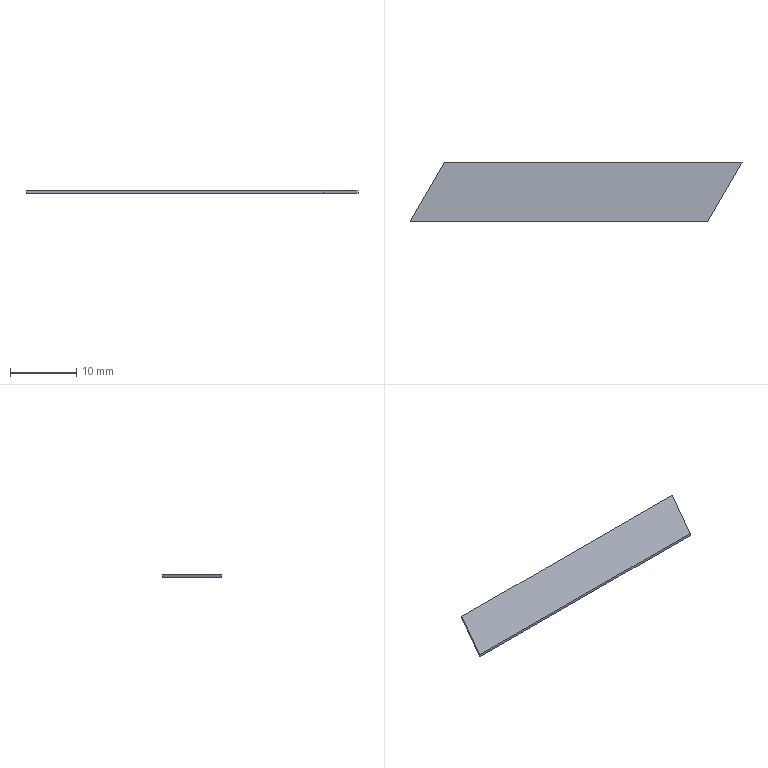Part | SolidWorks | features Extrusion 1 | 1 solid | 6 faces | box 50.196 x 9 x 0.4 mm | volume 162 mm3 | plane 6
STEP:
#1=CARTESIAN_POINT('',(5.196,9.,0.));
#2=VERTEX_POINT('',#1);
#3=CARTESIAN_POINT('',(0.,0.,0.));
#4=VERTEX_POINT('',#3);
#5=CARTESIAN_POINT('',(0.,0.,0.));
#6=DIRECTION('',(-0.5,-0.866,0.));
#7=VECTOR('',#6,1000.);
#8=LINE('',#5,#7);
#9=EDGE_CURVE('',#2,#4,#8,.T.);
#10=ORIENTED_EDGE('',*,*,#9,.T.);
#11=CARTESIAN_POINT('',(0.,0.,0.4));
#12=VERTEX_POINT('',#11);
#13=CARTESIAN_POINT('',(0.,0.,0.4));
#14=DIRECTION('',(0.,0.,-1.));
#15=VECTOR('',#14,1000.);
#16=LINE('',#13,#15);
#17=EDGE_CURVE('',#12,#4,#16,.T.);
#18=ORIENTED_EDGE('',*,*,#17,.F.);
#19=CARTESIAN_POINT('',(5.196,9.,0.4));
#20=VERTEX_POINT('',#19);
#21=CARTESIAN_POINT('',(0.,0.,0.4));
#22=DIRECTION('',(-0.5,-0.866,0.));
#23=VECTOR('',#22,1000.);
#24=LINE('',#21,#23);
#25=EDGE_CURVE('',#20,#12,#24,.T.);
#26=ORIENTED_EDGE('',*,*,#25,.F.);
#27=CARTESIAN_POINT('',(5.196,9.,0.4));
#28=DIRECTION('',(0.,0.,-1.));
#29=VECTOR('',#28,1000.);
#30=LINE('',#27,#29);
#31=EDGE_CURVE('',#20,#2,#30,.T.);
#32=ORIENTED_EDGE('',*,*,#31,.T.);
#33=EDGE_LOOP('',(#10,#18,#26,#32));
#34=FACE_OUTER_BOUND('',#33,.T.);
#35=CARTESIAN_POINT('',(0.,0.,0.4));
#36=DIRECTION('',(0.866,-0.5,0.));
#37=DIRECTION('',(0.5,0.866,0.));
#38=AXIS2_PLACEMENT_3D('',#35,#36,#37);
#39=PLANE('',#38);
#40=ADVANCED_FACE('',(#34),#39,.F.);
#41=CARTESIAN_POINT('',(45.,0.,0.));
#42=VERTEX_POINT('',#41);
#43=CARTESIAN_POINT('',(0.,0.,0.));
#44=DIRECTION('',(1.,0.,0.));
#45=VECTOR('',#44,1000.);
#46=LINE('',#43,#45);
#47=EDGE_CURVE('',#4,#42,#46,.T.);
#48=ORIENTED_EDGE('',*,*,#47,.T.);
#49=CARTESIAN_POINT('',(45.,0.,0.4));
#50=VERTEX_POINT('',#49);
#51=CARTESIAN_POINT('',(45.,0.,0.4));
#52=DIRECTION('',(0.,0.,-1.));
#53=VECTOR('',#52,1000.);
#54=LINE('',#51,#53);
#55=EDGE_CURVE('',#50,#42,#54,.T.);
#56=ORIENTED_EDGE('',*,*,#55,.F.);
#57=CARTESIAN_POINT('',(0.,0.,0.4));
#58=DIRECTION('',(1.,0.,0.));
#59=VECTOR('',#58,1000.);
#60=LINE('',#57,#59);
#61=EDGE_CURVE('',#12,#50,#60,.T.);
#62=ORIENTED_EDGE('',*,*,#61,.F.);
#63=ORIENTED_EDGE('',*,*,#17,.T.);
#64=EDGE_LOOP('',(#48,#56,#62,#63));
#65=FACE_OUTER_BOUND('',#64,.T.);
#66=CARTESIAN_POINT('',(0.,0.,0.4));
#67=DIRECTION('',(0.,1.,0.));
#68=DIRECTION('',(0.,0.,1.));
#69=AXIS2_PLACEMENT_3D('',#66,#67,#68);
#70=PLANE('',#69);
#71=ADVANCED_FACE('',(#65),#70,.F.);
#72=CARTESIAN_POINT('',(50.196,9.,0.));
#73=VERTEX_POINT('',#72);
#74=CARTESIAN_POINT('',(45.,0.,0.));
#75=DIRECTION('',(0.5,0.866,0.));
#76=VECTOR('',#75,1000.);
#77=LINE('',#74,#76);
#78=EDGE_CURVE('',#42,#73,#77,.T.);
#79=ORIENTED_EDGE('',*,*,#78,.T.);
#80=CARTESIAN_POINT('',(50.196,9.,0.4));
#81=VERTEX_POINT('',#80);
#82=CARTESIAN_POINT('',(50.196,9.,0.4));
#83=DIRECTION('',(0.,0.,-1.));
#84=VECTOR('',#83,1000.);
#85=LINE('',#82,#84);
#86=EDGE_CURVE('',#81,#73,#85,.T.);
#87=ORIENTED_EDGE('',*,*,#86,.F.);
#88=CARTESIAN_POINT('',(45.,0.,0.4));
#89=DIRECTION('',(0.5,0.866,0.));
#90=VECTOR('',#89,1000.);
#91=LINE('',#88,#90);
#92=EDGE_CURVE('',#50,#81,#91,.T.);
#93=ORIENTED_EDGE('',*,*,#92,.F.);
#94=ORIENTED_EDGE('',*,*,#55,.T.);
#95=EDGE_LOOP('',(#79,#87,#93,#94));
#96=FACE_OUTER_BOUND('',#95,.T.);
#97=CARTESIAN_POINT('',(45.,0.,0.4));
#98=DIRECTION('',(-0.866,0.5,0.));
#99=DIRECTION('',(-0.5,-0.866,0.));
#100=AXIS2_PLACEMENT_3D('',#97,#98,#99);
#101=PLANE('',#100);
#102=ADVANCED_FACE('',(#96),#101,.F.);
#103=CARTESIAN_POINT('',(5.196,9.,0.));
#104=DIRECTION('',(-1.,0.,0.));
#105=VECTOR('',#104,1000.);
#106=LINE('',#103,#105);
#107=EDGE_CURVE('',#73,#2,#106,.T.);
#108=ORIENTED_EDGE('',*,*,#107,.T.);
#109=ORIENTED_EDGE('',*,*,#31,.F.);
#110=CARTESIAN_POINT('',(5.196,9.,0.4));
#111=DIRECTION('',(-1.,0.,0.));
#112=VECTOR('',#111,1000.);
#113=LINE('',#110,#112);
#114=EDGE_CURVE('',#81,#20,#113,.T.);
#115=ORIENTED_EDGE('',*,*,#114,.F.);
#116=ORIENTED_EDGE('',*,*,#86,.T.);
#117=EDGE_LOOP('',(#108,#109,#115,#116));
#118=FACE_OUTER_BOUND('',#117,.T.);
#119=CARTESIAN_POINT('',(5.196,9.,0.4));
#120=DIRECTION('',(0.,-1.,0.));
#121=DIRECTION('',(0.,0.,-1.));
#122=AXIS2_PLACEMENT_3D('',#119,#120,#121);
#123=PLANE('',#122);
#124=ADVANCED_FACE('',(#118),#123,.F.);
#125=ORIENTED_EDGE('',*,*,#25,.T.);
#126=ORIENTED_EDGE('',*,*,#61,.T.);
#127=ORIENTED_EDGE('',*,*,#92,.T.);
#128=ORIENTED_EDGE('',*,*,#114,.T.);
#129=EDGE_LOOP('',(#125,#126,#127,#128));
#130=FACE_OUTER_BOUND('',#129,.T.);
#131=CARTESIAN_POINT('',(0.,0.,0.4));
#132=DIRECTION('',(0.,0.,-1.));
#133=DIRECTION('',(-1.,0.,0.));
#134=AXIS2_PLACEMENT_3D('',#131,#132,#133);
#135=PLANE('',#134);
#136=ADVANCED_FACE('',(#130),#135,.F.);
#137=ORIENTED_EDGE('',*,*,#9,.F.);
#138=ORIENTED_EDGE('',*,*,#107,.F.);
#139=ORIENTED_EDGE('',*,*,#78,.F.);
#140=ORIENTED_EDGE('',*,*,#47,.F.);
#141=EDGE_LOOP('',(#137,#138,#139,#140));
#142=FACE_OUTER_BOUND('',#141,.T.);
#143=CARTESIAN_POINT('',(0.,0.,0.));
#144=DIRECTION('',(0.,0.,-1.));
#145=DIRECTION('',(-1.,0.,0.));
#146=AXIS2_PLACEMENT_3D('',#143,#144,#145);
#147=PLANE('',#146);
#148=ADVANCED_FACE('',(#142),#147,.T.);
#149=CLOSED_SHELL('',(#40,#71,#102,#124,#136,#148));
#150=MANIFOLD_SOLID_BREP('',#149);
#151=CARTESIAN_POINT('',(0.,0.,0.));
#152=DIRECTION('',(0.,0.,1.));
#153=DIRECTION('',(1.,0.,0.));
#154=AXIS2_PLACEMENT_3D('',#151,#152,#153);
#155=(LENGTH_UNIT()NAMED_UNIT(*)SI_UNIT(.MILLI.,.METRE.));
#156=UNCERTAINTY_MEASURE_WITH_UNIT(LENGTH_MEASURE(0.00001),#155,'','');
#157=(NAMED_UNIT(*)PLANE_ANGLE_UNIT()SI_UNIT($,.RADIAN.));
#158=(NAMED_UNIT(*)SI_UNIT($,.STERADIAN.)SOLID_ANGLE_UNIT());
#159=(GEOMETRIC_REPRESENTATION_CONTEXT(3)GLOBAL_UNCERTAINTY_ASSIGNED_CONTEXT((#156))GLOBAL_UNIT_ASSIGNED_CONTEXT((#155,#157,#158))REPRESENTATION_CONTEXT('',''));
#160=ADVANCED_BREP_SHAPE_REPRESENTATION('',(#150,#154),#159);